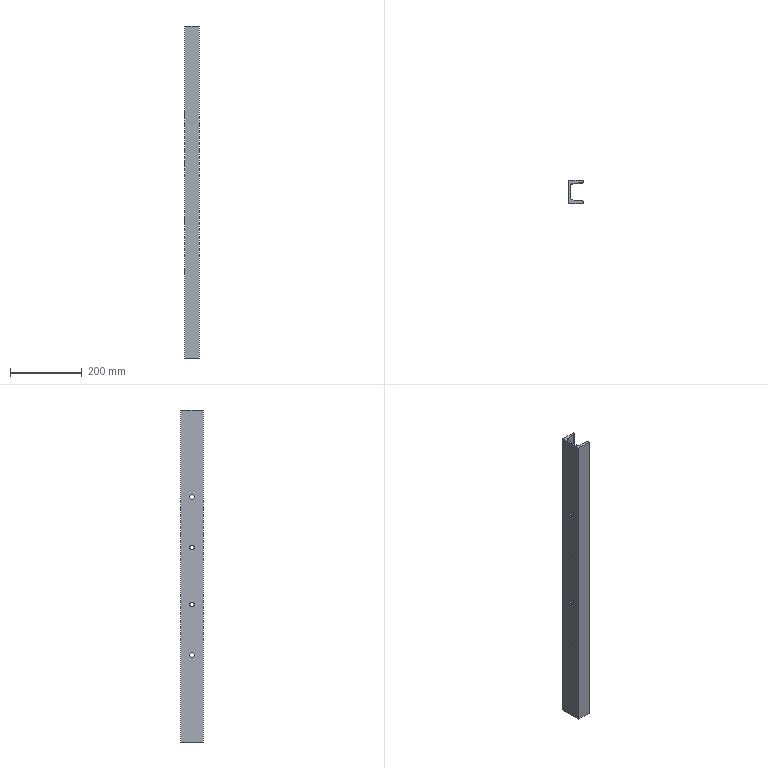Part | STEP file | 750038481 | 1 solid | 22 faces | box 40 x 63 x 924 mm | volume 778209 mm3 | cylinder 12 | plane 10 | commonest cylinder face diameters 12 x8 7.6 x2 15 x2
STEP:
#1=CARTESIAN_POINT('',(4.8,31.5,-86.));
#2=VERTEX_POINT('',#1);
#3=CARTESIAN_POINT('',(4.8,31.5,-74.));
#4=VERTEX_POINT('',#3);
#5=CARTESIAN_POINT('',(4.8,31.5,-80.));
#6=DIRECTION('',(-1.,0.,0.));
#7=DIRECTION('',(0.,0.,1.));
#8=AXIS2_PLACEMENT_3D('',#5,#6,#7);
#9=CIRCLE('',#8,6.);
#10=EDGE_CURVE('',#2,#4,#9,.T.);
#11=ORIENTED_EDGE('',*,*,#10,.F.);
#12=CARTESIAN_POINT('',(0.,31.5,-86.));
#13=VERTEX_POINT('',#12);
#14=CARTESIAN_POINT('',(279.,31.5,-86.));
#15=DIRECTION('',(-1.,0.,0.));
#16=VECTOR('',#15,1000.);
#17=LINE('',#14,#16);
#18=EDGE_CURVE('',#2,#13,#17,.T.);
#19=ORIENTED_EDGE('',*,*,#18,.T.);
#20=CARTESIAN_POINT('',(0.,31.5,-74.));
#21=VERTEX_POINT('',#20);
#22=CARTESIAN_POINT('',(0.,31.5,-80.));
#23=DIRECTION('',(-1.,0.,0.));
#24=DIRECTION('',(0.,0.,1.));
#25=AXIS2_PLACEMENT_3D('',#22,#23,#24);
#26=CIRCLE('',#25,6.);
#27=EDGE_CURVE('',#13,#21,#26,.T.);
#28=ORIENTED_EDGE('',*,*,#27,.T.);
#29=CARTESIAN_POINT('',(279.,31.5,-74.));
#30=DIRECTION('',(-1.,0.,0.));
#31=VECTOR('',#30,1000.);
#32=LINE('',#29,#31);
#33=EDGE_CURVE('',#4,#21,#32,.T.);
#34=ORIENTED_EDGE('',*,*,#33,.F.);
#35=EDGE_LOOP('',(#11,#19,#28,#34));
#36=FACE_OUTER_BOUND('',#35,.T.);
#37=CARTESIAN_POINT('',(279.,31.5,-80.));
#38=DIRECTION('',(-1.,0.,0.));
#39=DIRECTION('',(0.,0.,1.));
#40=AXIS2_PLACEMENT_3D('',#37,#38,#39);
#41=CYLINDRICAL_SURFACE('',#40,6.);
#42=ADVANCED_FACE('',(#36),#41,.F.);
#43=CARTESIAN_POINT('',(4.8,31.5,-226.));
#44=VERTEX_POINT('',#43);
#45=CARTESIAN_POINT('',(4.8,31.5,-214.));
#46=VERTEX_POINT('',#45);
#47=CARTESIAN_POINT('',(4.8,31.5,-220.));
#48=DIRECTION('',(-1.,0.,0.));
#49=DIRECTION('',(0.,0.,1.));
#50=AXIS2_PLACEMENT_3D('',#47,#48,#49);
#51=CIRCLE('',#50,6.);
#52=EDGE_CURVE('',#44,#46,#51,.T.);
#53=ORIENTED_EDGE('',*,*,#52,.F.);
#54=CARTESIAN_POINT('',(0.,31.5,-226.));
#55=VERTEX_POINT('',#54);
#56=CARTESIAN_POINT('',(279.,31.5,-226.));
#57=DIRECTION('',(-1.,0.,0.));
#58=VECTOR('',#57,1000.);
#59=LINE('',#56,#58);
#60=EDGE_CURVE('',#44,#55,#59,.T.);
#61=ORIENTED_EDGE('',*,*,#60,.T.);
#62=CARTESIAN_POINT('',(0.,31.5,-214.));
#63=VERTEX_POINT('',#62);
#64=CARTESIAN_POINT('',(0.,31.5,-220.));
#65=DIRECTION('',(-1.,0.,0.));
#66=DIRECTION('',(0.,0.,1.));
#67=AXIS2_PLACEMENT_3D('',#64,#65,#66);
#68=CIRCLE('',#67,6.);
#69=EDGE_CURVE('',#55,#63,#68,.T.);
#70=ORIENTED_EDGE('',*,*,#69,.T.);
#71=CARTESIAN_POINT('',(279.,31.5,-214.));
#72=DIRECTION('',(-1.,0.,0.));
#73=VECTOR('',#72,1000.);
#74=LINE('',#71,#73);
#75=EDGE_CURVE('',#46,#63,#74,.T.);
#76=ORIENTED_EDGE('',*,*,#75,.F.);
#77=EDGE_LOOP('',(#53,#61,#70,#76));
#78=FACE_OUTER_BOUND('',#77,.T.);
#79=CARTESIAN_POINT('',(279.,31.5,-220.));
#80=DIRECTION('',(-1.,0.,0.));
#81=DIRECTION('',(0.,0.,1.));
#82=AXIS2_PLACEMENT_3D('',#79,#80,#81);
#83=CYLINDRICAL_SURFACE('',#82,6.);
#84=ADVANCED_FACE('',(#78),#83,.F.);
#85=CARTESIAN_POINT('',(4.8,31.5,74.));
#86=VERTEX_POINT('',#85);
#87=CARTESIAN_POINT('',(4.8,31.5,86.));
#88=VERTEX_POINT('',#87);
#89=CARTESIAN_POINT('',(4.8,31.5,80.));
#90=DIRECTION('',(-1.,0.,0.));
#91=DIRECTION('',(0.,0.,1.));
#92=AXIS2_PLACEMENT_3D('',#89,#90,#91);
#93=CIRCLE('',#92,6.);
#94=EDGE_CURVE('',#86,#88,#93,.T.);
#95=ORIENTED_EDGE('',*,*,#94,.F.);
#96=CARTESIAN_POINT('',(0.,31.5,74.));
#97=VERTEX_POINT('',#96);
#98=CARTESIAN_POINT('',(279.,31.5,74.));
#99=DIRECTION('',(-1.,0.,0.));
#100=VECTOR('',#99,1000.);
#101=LINE('',#98,#100);
#102=EDGE_CURVE('',#86,#97,#101,.T.);
#103=ORIENTED_EDGE('',*,*,#102,.T.);
#104=CARTESIAN_POINT('',(0.,31.5,86.));
#105=VERTEX_POINT('',#104);
#106=CARTESIAN_POINT('',(0.,31.5,80.));
#107=DIRECTION('',(-1.,0.,0.));
#108=DIRECTION('',(0.,0.,1.));
#109=AXIS2_PLACEMENT_3D('',#106,#107,#108);
#110=CIRCLE('',#109,6.);
#111=EDGE_CURVE('',#97,#105,#110,.T.);
#112=ORIENTED_EDGE('',*,*,#111,.T.);
#113=CARTESIAN_POINT('',(279.,31.5,86.));
#114=DIRECTION('',(-1.,0.,0.));
#115=VECTOR('',#114,1000.);
#116=LINE('',#113,#115);
#117=EDGE_CURVE('',#88,#105,#116,.T.);
#118=ORIENTED_EDGE('',*,*,#117,.F.);
#119=EDGE_LOOP('',(#95,#103,#112,#118));
#120=FACE_OUTER_BOUND('',#119,.T.);
#121=CARTESIAN_POINT('',(279.,31.5,80.));
#122=DIRECTION('',(-1.,0.,0.));
#123=DIRECTION('',(0.,0.,1.));
#124=AXIS2_PLACEMENT_3D('',#121,#122,#123);
#125=CYLINDRICAL_SURFACE('',#124,6.);
#126=ADVANCED_FACE('',(#120),#125,.F.);
#127=CARTESIAN_POINT('',(4.8,31.5,214.));
#128=VERTEX_POINT('',#127);
#129=CARTESIAN_POINT('',(4.8,31.5,226.));
#130=VERTEX_POINT('',#129);
#131=CARTESIAN_POINT('',(4.8,31.5,220.));
#132=DIRECTION('',(-1.,0.,0.));
#133=DIRECTION('',(0.,0.,1.));
#134=AXIS2_PLACEMENT_3D('',#131,#132,#133);
#135=CIRCLE('',#134,6.);
#136=EDGE_CURVE('',#128,#130,#135,.T.);
#137=ORIENTED_EDGE('',*,*,#136,.F.);
#138=CARTESIAN_POINT('',(0.,31.5,214.));
#139=VERTEX_POINT('',#138);
#140=CARTESIAN_POINT('',(279.,31.5,214.));
#141=DIRECTION('',(-1.,0.,0.));
#142=VECTOR('',#141,1000.);
#143=LINE('',#140,#142);
#144=EDGE_CURVE('',#128,#139,#143,.T.);
#145=ORIENTED_EDGE('',*,*,#144,.T.);
#146=CARTESIAN_POINT('',(0.,31.5,226.));
#147=VERTEX_POINT('',#146);
#148=CARTESIAN_POINT('',(0.,31.5,220.));
#149=DIRECTION('',(-1.,0.,0.));
#150=DIRECTION('',(0.,0.,1.));
#151=AXIS2_PLACEMENT_3D('',#148,#149,#150);
#152=CIRCLE('',#151,6.);
#153=EDGE_CURVE('',#139,#147,#152,.T.);
#154=ORIENTED_EDGE('',*,*,#153,.T.);
#155=CARTESIAN_POINT('',(279.,31.5,226.));
#156=DIRECTION('',(-1.,0.,0.));
#157=VECTOR('',#156,1000.);
#158=LINE('',#155,#157);
#159=EDGE_CURVE('',#130,#147,#158,.T.);
#160=ORIENTED_EDGE('',*,*,#159,.F.);
#161=EDGE_LOOP('',(#137,#145,#154,#160));
#162=FACE_OUTER_BOUND('',#161,.T.);
#163=CARTESIAN_POINT('',(279.,31.5,220.));
#164=DIRECTION('',(-1.,0.,0.));
#165=DIRECTION('',(0.,0.,1.));
#166=AXIS2_PLACEMENT_3D('',#163,#164,#165);
#167=CYLINDRICAL_SURFACE('',#166,6.);
#168=ADVANCED_FACE('',(#162),#167,.F.);
#169=CARTESIAN_POINT('',(0.,31.5,-80.));
#170=DIRECTION('',(-1.,0.,0.));
#171=DIRECTION('',(0.,0.,1.));
#172=AXIS2_PLACEMENT_3D('',#169,#170,#171);
#173=CIRCLE('',#172,6.);
#174=EDGE_CURVE('',#21,#13,#173,.T.);
#175=ORIENTED_EDGE('',*,*,#174,.F.);
#176=ORIENTED_EDGE('',*,*,#27,.F.);
#177=EDGE_LOOP('',(#175,#176));
#178=FACE_BOUND('',#177,.T.);
#179=CARTESIAN_POINT('',(0.,31.5,-220.));
#180=DIRECTION('',(-1.,0.,0.));
#181=DIRECTION('',(0.,0.,1.));
#182=AXIS2_PLACEMENT_3D('',#179,#180,#181);
#183=CIRCLE('',#182,6.);
#184=EDGE_CURVE('',#63,#55,#183,.T.);
#185=ORIENTED_EDGE('',*,*,#184,.F.);
#186=ORIENTED_EDGE('',*,*,#69,.F.);
#187=EDGE_LOOP('',(#185,#186));
#188=FACE_BOUND('',#187,.T.);
#189=CARTESIAN_POINT('',(0.,0.,462.));
#190=VERTEX_POINT('',#189);
#191=CARTESIAN_POINT('',(0.,0.,-462.));
#192=VERTEX_POINT('',#191);
#193=CARTESIAN_POINT('',(0.,0.,462.));
#194=DIRECTION('',(0.,0.,-1.));
#195=VECTOR('',#194,1000.);
#196=LINE('',#193,#195);
#197=EDGE_CURVE('',#190,#192,#196,.T.);
#198=ORIENTED_EDGE('',*,*,#197,.F.);
#199=CARTESIAN_POINT('',(0.,63.,462.));
#200=VERTEX_POINT('',#199);
#201=CARTESIAN_POINT('',(0.,63.,462.));
#202=DIRECTION('',(0.,-1.,0.));
#203=VECTOR('',#202,1000.);
#204=LINE('',#201,#203);
#205=EDGE_CURVE('',#200,#190,#204,.T.);
#206=ORIENTED_EDGE('',*,*,#205,.F.);
#207=CARTESIAN_POINT('',(0.,63.,-462.));
#208=VERTEX_POINT('',#207);
#209=CARTESIAN_POINT('',(0.,63.,462.));
#210=DIRECTION('',(0.,0.,1.));
#211=VECTOR('',#210,1000.);
#212=LINE('',#209,#211);
#213=EDGE_CURVE('',#208,#200,#212,.T.);
#214=ORIENTED_EDGE('',*,*,#213,.F.);
#215=CARTESIAN_POINT('',(0.,63.,-462.));
#216=DIRECTION('',(0.,1.,0.));
#217=VECTOR('',#216,1000.);
#218=LINE('',#215,#217);
#219=EDGE_CURVE('',#192,#208,#218,.T.);
#220=ORIENTED_EDGE('',*,*,#219,.F.);
#221=EDGE_LOOP('',(#198,#206,#214,#220));
#222=FACE_OUTER_BOUND('',#221,.T.);
#223=CARTESIAN_POINT('',(0.,31.5,80.));
#224=DIRECTION('',(-1.,0.,0.));
#225=DIRECTION('',(0.,0.,1.));
#226=AXIS2_PLACEMENT_3D('',#223,#224,#225);
#227=CIRCLE('',#226,6.);
#228=EDGE_CURVE('',#105,#97,#227,.T.);
#229=ORIENTED_EDGE('',*,*,#228,.F.);
#230=ORIENTED_EDGE('',*,*,#111,.F.);
#231=EDGE_LOOP('',(#229,#230));
#232=FACE_BOUND('',#231,.T.);
#233=CARTESIAN_POINT('',(0.,31.5,220.));
#234=DIRECTION('',(-1.,0.,0.));
#235=DIRECTION('',(0.,0.,1.));
#236=AXIS2_PLACEMENT_3D('',#233,#234,#235);
#237=CIRCLE('',#236,6.);
#238=EDGE_CURVE('',#147,#139,#237,.T.);
#239=ORIENTED_EDGE('',*,*,#238,.F.);
#240=ORIENTED_EDGE('',*,*,#153,.F.);
#241=EDGE_LOOP('',(#239,#240));
#242=FACE_BOUND('',#241,.T.);
#243=CARTESIAN_POINT('',(0.,63.,462.));
#244=DIRECTION('',(1.,0.,0.));
#245=DIRECTION('',(0.,0.,-1.));
#246=AXIS2_PLACEMENT_3D('',#243,#244,#245);
#247=PLANE('',#246);
#248=ADVANCED_FACE('',(#178,#188,#222,#232,#242),#247,.F.);
#249=ORIENTED_EDGE('',*,*,#18,.F.);
#250=CARTESIAN_POINT('',(4.8,31.5,-80.));
#251=DIRECTION('',(-1.,0.,0.));
#252=DIRECTION('',(0.,0.,1.));
#253=AXIS2_PLACEMENT_3D('',#250,#251,#252);
#254=CIRCLE('',#253,6.);
#255=EDGE_CURVE('',#4,#2,#254,.T.);
#256=ORIENTED_EDGE('',*,*,#255,.F.);
#257=ORIENTED_EDGE('',*,*,#33,.T.);
#258=ORIENTED_EDGE('',*,*,#174,.T.);
#259=EDGE_LOOP('',(#249,#256,#257,#258));
#260=FACE_OUTER_BOUND('',#259,.T.);
#261=CARTESIAN_POINT('',(279.,31.5,-80.));
#262=DIRECTION('',(-1.,0.,0.));
#263=DIRECTION('',(0.,0.,1.));
#264=AXIS2_PLACEMENT_3D('',#261,#262,#263);
#265=CYLINDRICAL_SURFACE('',#264,6.);
#266=ADVANCED_FACE('',(#260),#265,.F.);
#267=ORIENTED_EDGE('',*,*,#60,.F.);
#268=CARTESIAN_POINT('',(4.8,31.5,-220.));
#269=DIRECTION('',(-1.,0.,0.));
#270=DIRECTION('',(0.,0.,1.));
#271=AXIS2_PLACEMENT_3D('',#268,#269,#270);
#272=CIRCLE('',#271,6.);
#273=EDGE_CURVE('',#46,#44,#272,.T.);
#274=ORIENTED_EDGE('',*,*,#273,.F.);
#275=ORIENTED_EDGE('',*,*,#75,.T.);
#276=ORIENTED_EDGE('',*,*,#184,.T.);
#277=EDGE_LOOP('',(#267,#274,#275,#276));
#278=FACE_OUTER_BOUND('',#277,.T.);
#279=CARTESIAN_POINT('',(279.,31.5,-220.));
#280=DIRECTION('',(-1.,0.,0.));
#281=DIRECTION('',(0.,0.,1.));
#282=AXIS2_PLACEMENT_3D('',#279,#280,#281);
#283=CYLINDRICAL_SURFACE('',#282,6.);
#284=ADVANCED_FACE('',(#278),#283,.F.);
#285=CARTESIAN_POINT('',(40.,63.,-462.));
#286=VERTEX_POINT('',#285);
#287=CARTESIAN_POINT('',(36.2,63.,-462.));
#288=DIRECTION('',(-1.,0.,0.));
#289=VECTOR('',#288,1000.);
#290=LINE('',#287,#289);
#291=EDGE_CURVE('',#286,#208,#290,.T.);
#292=ORIENTED_EDGE('',*,*,#291,.F.);
#293=CARTESIAN_POINT('',(40.,60.699,-462.));
#294=VERTEX_POINT('',#293);
#295=CARTESIAN_POINT('',(40.,2.301,-462.));
#296=DIRECTION('',(0.,1.,0.));
#297=VECTOR('',#296,1000.);
#298=LINE('',#295,#297);
#299=EDGE_CURVE('',#294,#286,#298,.T.);
#300=ORIENTED_EDGE('',*,*,#299,.F.);
#301=CARTESIAN_POINT('',(36.578,56.918,-462.));
#302=VERTEX_POINT('',#301);
#303=CARTESIAN_POINT('',(36.2,60.699,-462.));
#304=DIRECTION('',(0.,0.,1.));
#305=DIRECTION('',(-1.,0.,0.));
#306=AXIS2_PLACEMENT_3D('',#303,#304,#305);
#307=CIRCLE('',#306,3.8);
#308=EDGE_CURVE('',#302,#294,#307,.T.);
#309=ORIENTED_EDGE('',*,*,#308,.F.);
#310=CARTESIAN_POINT('',(11.554,54.415,-462.));
#311=VERTEX_POINT('',#310);
#312=CARTESIAN_POINT('',(11.554,54.415,-462.));
#313=DIRECTION('',(0.995,0.0995,0.));
#314=VECTOR('',#313,1000.);
#315=LINE('',#312,#314);
#316=EDGE_CURVE('',#311,#302,#315,.T.);
#317=ORIENTED_EDGE('',*,*,#316,.F.);
#318=CARTESIAN_POINT('',(4.8,46.953,-462.));
#319=VERTEX_POINT('',#318);
#320=CARTESIAN_POINT('',(12.3,46.953,-462.));
#321=DIRECTION('',(0.,0.,-1.));
#322=DIRECTION('',(-1.,0.,0.));
#323=AXIS2_PLACEMENT_3D('',#320,#321,#322);
#324=CIRCLE('',#323,7.5);
#325=EDGE_CURVE('',#319,#311,#324,.T.);
#326=ORIENTED_EDGE('',*,*,#325,.F.);
#327=CARTESIAN_POINT('',(4.8,16.047,-462.));
#328=VERTEX_POINT('',#327);
#329=CARTESIAN_POINT('',(4.8,2.301,-462.));
#330=DIRECTION('',(0.,1.,0.));
#331=VECTOR('',#330,1000.);
#332=LINE('',#329,#331);
#333=EDGE_CURVE('',#328,#319,#332,.T.);
#334=ORIENTED_EDGE('',*,*,#333,.F.);
#335=CARTESIAN_POINT('',(11.554,8.585,-462.));
#336=VERTEX_POINT('',#335);
#337=CARTESIAN_POINT('',(12.3,16.047,-462.));
#338=DIRECTION('',(0.,0.,-1.));
#339=DIRECTION('',(-1.,0.,0.));
#340=AXIS2_PLACEMENT_3D('',#337,#338,#339);
#341=CIRCLE('',#340,7.5);
#342=EDGE_CURVE('',#336,#328,#341,.T.);
#343=ORIENTED_EDGE('',*,*,#342,.F.);
#344=CARTESIAN_POINT('',(36.578,6.082,-462.));
#345=VERTEX_POINT('',#344);
#346=CARTESIAN_POINT('',(36.578,6.082,-462.));
#347=DIRECTION('',(-0.995,0.0995,0.));
#348=VECTOR('',#347,1000.);
#349=LINE('',#346,#348);
#350=EDGE_CURVE('',#345,#336,#349,.T.);
#351=ORIENTED_EDGE('',*,*,#350,.F.);
#352=CARTESIAN_POINT('',(40.,2.301,-462.));
#353=VERTEX_POINT('',#352);
#354=CARTESIAN_POINT('',(36.2,2.301,-462.));
#355=DIRECTION('',(0.,0.,1.));
#356=DIRECTION('',(-1.,0.,0.));
#357=AXIS2_PLACEMENT_3D('',#354,#355,#356);
#358=CIRCLE('',#357,3.8);
#359=EDGE_CURVE('',#353,#345,#358,.T.);
#360=ORIENTED_EDGE('',*,*,#359,.F.);
#361=CARTESIAN_POINT('',(40.,0.,-462.));
#362=VERTEX_POINT('',#361);
#363=CARTESIAN_POINT('',(40.,2.301,-462.));
#364=DIRECTION('',(0.,1.,0.));
#365=VECTOR('',#364,1000.);
#366=LINE('',#363,#365);
#367=EDGE_CURVE('',#362,#353,#366,.T.);
#368=ORIENTED_EDGE('',*,*,#367,.F.);
#369=CARTESIAN_POINT('',(36.2,0.,-462.));
#370=DIRECTION('',(1.,0.,0.));
#371=VECTOR('',#370,1000.);
#372=LINE('',#369,#371);
#373=EDGE_CURVE('',#192,#362,#372,.T.);
#374=ORIENTED_EDGE('',*,*,#373,.F.);
#375=ORIENTED_EDGE('',*,*,#219,.T.);
#376=EDGE_LOOP('',(#292,#300,#309,#317,#326,#334,#343,#351,#360,#368,#374,#375));
#377=FACE_OUTER_BOUND('',#376,.T.);
#378=CARTESIAN_POINT('',(36.2,2.301,-462.));
#379=DIRECTION('',(0.,0.,1.));
#380=DIRECTION('',(1.,0.,0.));
#381=AXIS2_PLACEMENT_3D('',#378,#379,#380);
#382=PLANE('',#381);
#383=ADVANCED_FACE('',(#377),#382,.F.);
#384=CARTESIAN_POINT('',(40.,0.,462.));
#385=VERTEX_POINT('',#384);
#386=CARTESIAN_POINT('',(40.,0.,462.));
#387=DIRECTION('',(0.,0.,-1.));
#388=VECTOR('',#387,1000.);
#389=LINE('',#386,#388);
#390=EDGE_CURVE('',#385,#362,#389,.T.);
#391=ORIENTED_EDGE('',*,*,#390,.F.);
#392=CARTESIAN_POINT('',(0.,0.,462.));
#393=DIRECTION('',(1.,0.,0.));
#394=VECTOR('',#393,1000.);
#395=LINE('',#392,#394);
#396=EDGE_CURVE('',#190,#385,#395,.T.);
#397=ORIENTED_EDGE('',*,*,#396,.F.);
#398=ORIENTED_EDGE('',*,*,#197,.T.);
#399=ORIENTED_EDGE('',*,*,#373,.T.);
#400=EDGE_LOOP('',(#391,#397,#398,#399));
#401=FACE_OUTER_BOUND('',#400,.T.);
#402=CARTESIAN_POINT('',(0.,0.,462.));
#403=DIRECTION('',(0.,1.,0.));
#404=DIRECTION('',(0.,0.,1.));
#405=AXIS2_PLACEMENT_3D('',#402,#403,#404);
#406=PLANE('',#405);
#407=ADVANCED_FACE('',(#401),#406,.F.);
#408=CARTESIAN_POINT('',(40.,60.699,462.));
#409=VERTEX_POINT('',#408);
#410=CARTESIAN_POINT('',(40.,63.,462.));
#411=VERTEX_POINT('',#410);
#412=CARTESIAN_POINT('',(40.,2.301,462.));
#413=DIRECTION('',(0.,1.,0.));
#414=VECTOR('',#413,1000.);
#415=LINE('',#412,#414);
#416=EDGE_CURVE('',#409,#411,#415,.T.);
#417=ORIENTED_EDGE('',*,*,#416,.T.);
#418=CARTESIAN_POINT('',(36.2,63.,462.));
#419=DIRECTION('',(-1.,0.,0.));
#420=VECTOR('',#419,1000.);
#421=LINE('',#418,#420);
#422=EDGE_CURVE('',#411,#200,#421,.T.);
#423=ORIENTED_EDGE('',*,*,#422,.T.);
#424=ORIENTED_EDGE('',*,*,#205,.T.);
#425=ORIENTED_EDGE('',*,*,#396,.T.);
#426=CARTESIAN_POINT('',(40.,2.301,462.));
#427=VERTEX_POINT('',#426);
#428=CARTESIAN_POINT('',(40.,2.301,462.));
#429=DIRECTION('',(0.,1.,0.));
#430=VECTOR('',#429,1000.);
#431=LINE('',#428,#430);
#432=EDGE_CURVE('',#385,#427,#431,.T.);
#433=ORIENTED_EDGE('',*,*,#432,.T.);
#434=CARTESIAN_POINT('',(36.578,6.082,462.));
#435=VERTEX_POINT('',#434);
#436=CARTESIAN_POINT('',(36.2,2.301,462.));
#437=DIRECTION('',(0.,0.,1.));
#438=DIRECTION('',(-1.,0.,0.));
#439=AXIS2_PLACEMENT_3D('',#436,#437,#438);
#440=CIRCLE('',#439,3.8);
#441=EDGE_CURVE('',#427,#435,#440,.T.);
#442=ORIENTED_EDGE('',*,*,#441,.T.);
#443=CARTESIAN_POINT('',(11.554,8.585,462.));
#444=VERTEX_POINT('',#443);
#445=CARTESIAN_POINT('',(36.578,6.082,462.));
#446=DIRECTION('',(-0.995,0.0995,0.));
#447=VECTOR('',#446,1000.);
#448=LINE('',#445,#447);
#449=EDGE_CURVE('',#435,#444,#448,.T.);
#450=ORIENTED_EDGE('',*,*,#449,.T.);
#451=CARTESIAN_POINT('',(4.8,16.047,462.));
#452=VERTEX_POINT('',#451);
#453=CARTESIAN_POINT('',(12.3,16.047,462.));
#454=DIRECTION('',(0.,0.,-1.));
#455=DIRECTION('',(-1.,0.,0.));
#456=AXIS2_PLACEMENT_3D('',#453,#454,#455);
#457=CIRCLE('',#456,7.5);
#458=EDGE_CURVE('',#444,#452,#457,.T.);
#459=ORIENTED_EDGE('',*,*,#458,.T.);
#460=CARTESIAN_POINT('',(4.8,46.953,462.));
#461=VERTEX_POINT('',#460);
#462=CARTESIAN_POINT('',(4.8,2.301,462.));
#463=DIRECTION('',(0.,1.,0.));
#464=VECTOR('',#463,1000.);
#465=LINE('',#462,#464);
#466=EDGE_CURVE('',#452,#461,#465,.T.);
#467=ORIENTED_EDGE('',*,*,#466,.T.);
#468=CARTESIAN_POINT('',(11.554,54.415,462.));
#469=VERTEX_POINT('',#468);
#470=CARTESIAN_POINT('',(12.3,46.953,462.));
#471=DIRECTION('',(0.,0.,-1.));
#472=DIRECTION('',(-1.,0.,0.));
#473=AXIS2_PLACEMENT_3D('',#470,#471,#472);
#474=CIRCLE('',#473,7.5);
#475=EDGE_CURVE('',#461,#469,#474,.T.);
#476=ORIENTED_EDGE('',*,*,#475,.T.);
#477=CARTESIAN_POINT('',(36.578,56.918,462.));
#478=VERTEX_POINT('',#477);
#479=CARTESIAN_POINT('',(11.554,54.415,462.));
#480=DIRECTION('',(0.995,0.0995,0.));
#481=VECTOR('',#480,1000.);
#482=LINE('',#479,#481);
#483=EDGE_CURVE('',#469,#478,#482,.T.);
#484=ORIENTED_EDGE('',*,*,#483,.T.);
#485=CARTESIAN_POINT('',(36.2,60.699,462.));
#486=DIRECTION('',(0.,0.,1.));
#487=DIRECTION('',(-1.,0.,0.));
#488=AXIS2_PLACEMENT_3D('',#485,#486,#487);
#489=CIRCLE('',#488,3.8);
#490=EDGE_CURVE('',#478,#409,#489,.T.);
#491=ORIENTED_EDGE('',*,*,#490,.T.);
#492=EDGE_LOOP('',(#417,#423,#424,#425,#433,#442,#450,#459,#467,#476,#484,#491));
#493=FACE_OUTER_BOUND('',#492,.T.);
#494=CARTESIAN_POINT('',(36.2,2.301,462.));
#495=DIRECTION('',(0.,0.,1.));
#496=DIRECTION('',(1.,0.,0.));
#497=AXIS2_PLACEMENT_3D('',#494,#495,#496);
#498=PLANE('',#497);
#499=ADVANCED_FACE('',(#493),#498,.T.);
#500=ORIENTED_EDGE('',*,*,#213,.T.);
#501=ORIENTED_EDGE('',*,*,#422,.F.);
#502=CARTESIAN_POINT('',(40.,63.,462.));
#503=DIRECTION('',(0.,0.,1.));
#504=VECTOR('',#503,1000.);
#505=LINE('',#502,#504);
#506=EDGE_CURVE('',#286,#411,#505,.T.);
#507=ORIENTED_EDGE('',*,*,#506,.F.);
#508=ORIENTED_EDGE('',*,*,#291,.T.);
#509=EDGE_LOOP('',(#500,#501,#507,#508));
#510=FACE_OUTER_BOUND('',#509,.T.);
#511=CARTESIAN_POINT('',(40.,63.,462.));
#512=DIRECTION('',(0.,-1.,0.));
#513=DIRECTION('',(0.,0.,-1.));
#514=AXIS2_PLACEMENT_3D('',#511,#512,#513);
#515=PLANE('',#514);
#516=ADVANCED_FACE('',(#510),#515,.F.);
#517=ORIENTED_EDGE('',*,*,#102,.F.);
#518=CARTESIAN_POINT('',(4.8,31.5,80.));
#519=DIRECTION('',(-1.,0.,0.));
#520=DIRECTION('',(0.,0.,1.));
#521=AXIS2_PLACEMENT_3D('',#518,#519,#520);
#522=CIRCLE('',#521,6.);
#523=EDGE_CURVE('',#88,#86,#522,.T.);
#524=ORIENTED_EDGE('',*,*,#523,.F.);
#525=ORIENTED_EDGE('',*,*,#117,.T.);
#526=ORIENTED_EDGE('',*,*,#228,.T.);
#527=EDGE_LOOP('',(#517,#524,#525,#526));
#528=FACE_OUTER_BOUND('',#527,.T.);
#529=CARTESIAN_POINT('',(279.,31.5,80.));
#530=DIRECTION('',(-1.,0.,0.));
#531=DIRECTION('',(0.,0.,1.));
#532=AXIS2_PLACEMENT_3D('',#529,#530,#531);
#533=CYLINDRICAL_SURFACE('',#532,6.);
#534=ADVANCED_FACE('',(#528),#533,.F.);
#535=ORIENTED_EDGE('',*,*,#144,.F.);
#536=CARTESIAN_POINT('',(4.8,31.5,220.));
#537=DIRECTION('',(-1.,0.,0.));
#538=DIRECTION('',(0.,0.,1.));
#539=AXIS2_PLACEMENT_3D('',#536,#537,#538);
#540=CIRCLE('',#539,6.);
#541=EDGE_CURVE('',#130,#128,#540,.T.);
#542=ORIENTED_EDGE('',*,*,#541,.F.);
#543=ORIENTED_EDGE('',*,*,#159,.T.);
#544=ORIENTED_EDGE('',*,*,#238,.T.);
#545=EDGE_LOOP('',(#535,#542,#543,#544));
#546=FACE_OUTER_BOUND('',#545,.T.);
#547=CARTESIAN_POINT('',(279.,31.5,220.));
#548=DIRECTION('',(-1.,0.,0.));
#549=DIRECTION('',(0.,0.,1.));
#550=AXIS2_PLACEMENT_3D('',#547,#548,#549);
#551=CYLINDRICAL_SURFACE('',#550,6.);
#552=ADVANCED_FACE('',(#546),#551,.F.);
#553=ORIENTED_EDGE('',*,*,#255,.T.);
#554=ORIENTED_EDGE('',*,*,#10,.T.);
#555=EDGE_LOOP('',(#553,#554));
#556=FACE_BOUND('',#555,.T.);
#557=CARTESIAN_POINT('',(4.8,46.953,462.));
#558=DIRECTION('',(0.,0.,-1.));
#559=VECTOR('',#558,1000.);
#560=LINE('',#557,#559);
#561=EDGE_CURVE('',#461,#319,#560,.T.);
#562=ORIENTED_EDGE('',*,*,#561,.F.);
#563=ORIENTED_EDGE('',*,*,#466,.F.);
#564=CARTESIAN_POINT('',(4.8,16.047,462.));
#565=DIRECTION('',(0.,0.,1.));
#566=VECTOR('',#565,1000.);
#567=LINE('',#564,#566);
#568=EDGE_CURVE('',#328,#452,#567,.T.);
#569=ORIENTED_EDGE('',*,*,#568,.F.);
#570=ORIENTED_EDGE('',*,*,#333,.T.);
#571=EDGE_LOOP('',(#562,#563,#569,#570));
#572=FACE_OUTER_BOUND('',#571,.T.);
#573=ORIENTED_EDGE('',*,*,#523,.T.);
#574=ORIENTED_EDGE('',*,*,#94,.T.);
#575=EDGE_LOOP('',(#573,#574));
#576=FACE_BOUND('',#575,.T.);
#577=ORIENTED_EDGE('',*,*,#273,.T.);
#578=ORIENTED_EDGE('',*,*,#52,.T.);
#579=EDGE_LOOP('',(#577,#578));
#580=FACE_BOUND('',#579,.T.);
#581=ORIENTED_EDGE('',*,*,#541,.T.);
#582=ORIENTED_EDGE('',*,*,#136,.T.);
#583=EDGE_LOOP('',(#581,#582));
#584=FACE_BOUND('',#583,.T.);
#585=CARTESIAN_POINT('',(4.8,16.047,462.));
#586=DIRECTION('',(-1.,0.,0.));
#587=DIRECTION('',(0.,-1.,0.));
#588=AXIS2_PLACEMENT_3D('',#585,#586,#587);
#589=PLANE('',#588);
#590=ADVANCED_FACE('',(#556,#572,#576,#580,#584),#589,.F.);
#591=ORIENTED_EDGE('',*,*,#506,.T.);
#592=ORIENTED_EDGE('',*,*,#416,.F.);
#593=CARTESIAN_POINT('',(40.,60.699,462.));
#594=DIRECTION('',(0.,0.,1.));
#595=VECTOR('',#594,1000.);
#596=LINE('',#593,#595);
#597=EDGE_CURVE('',#294,#409,#596,.T.);
#598=ORIENTED_EDGE('',*,*,#597,.F.);
#599=ORIENTED_EDGE('',*,*,#299,.T.);
#600=EDGE_LOOP('',(#591,#592,#598,#599));
#601=FACE_OUTER_BOUND('',#600,.T.);
#602=CARTESIAN_POINT('',(40.,60.699,462.));
#603=DIRECTION('',(-1.,0.,0.));
#604=DIRECTION('',(0.,-1.,0.));
#605=AXIS2_PLACEMENT_3D('',#602,#603,#604);
#606=PLANE('',#605);
#607=ADVANCED_FACE('',(#601),#606,.F.);
#608=ORIENTED_EDGE('',*,*,#490,.F.);
#609=CARTESIAN_POINT('',(36.578,56.918,462.));
#610=DIRECTION('',(0.,0.,-1.));
#611=VECTOR('',#610,1000.);
#612=LINE('',#609,#611);
#613=EDGE_CURVE('',#478,#302,#612,.T.);
#614=ORIENTED_EDGE('',*,*,#613,.T.);
#615=ORIENTED_EDGE('',*,*,#308,.T.);
#616=ORIENTED_EDGE('',*,*,#597,.T.);
#617=EDGE_LOOP('',(#608,#614,#615,#616));
#618=FACE_OUTER_BOUND('',#617,.T.);
#619=CARTESIAN_POINT('',(36.2,60.699,462.));
#620=DIRECTION('',(0.,0.,-1.));
#621=DIRECTION('',(-1.,0.,0.));
#622=AXIS2_PLACEMENT_3D('',#619,#620,#621);
#623=CYLINDRICAL_SURFACE('',#622,3.8);
#624=ADVANCED_FACE('',(#618),#623,.T.);
#625=ORIENTED_EDGE('',*,*,#613,.F.);
#626=ORIENTED_EDGE('',*,*,#483,.F.);
#627=CARTESIAN_POINT('',(11.554,54.415,462.));
#628=DIRECTION('',(0.,0.,1.));
#629=VECTOR('',#628,1000.);
#630=LINE('',#627,#629);
#631=EDGE_CURVE('',#311,#469,#630,.T.);
#632=ORIENTED_EDGE('',*,*,#631,.F.);
#633=ORIENTED_EDGE('',*,*,#316,.T.);
#634=EDGE_LOOP('',(#625,#626,#632,#633));
#635=FACE_OUTER_BOUND('',#634,.T.);
#636=CARTESIAN_POINT('',(11.554,54.415,462.));
#637=DIRECTION('',(-0.0995,0.995,0.));
#638=DIRECTION('',(-0.995,-0.0995,0.));
#639=AXIS2_PLACEMENT_3D('',#636,#637,#638);
#640=PLANE('',#639);
#641=ADVANCED_FACE('',(#635),#640,.F.);
#642=ORIENTED_EDGE('',*,*,#631,.T.);
#643=ORIENTED_EDGE('',*,*,#475,.F.);
#644=ORIENTED_EDGE('',*,*,#561,.T.);
#645=ORIENTED_EDGE('',*,*,#325,.T.);
#646=EDGE_LOOP('',(#642,#643,#644,#645));
#647=FACE_OUTER_BOUND('',#646,.T.);
#648=CARTESIAN_POINT('',(12.3,46.953,462.));
#649=DIRECTION('',(0.,0.,-1.));
#650=DIRECTION('',(-1.,0.,0.));
#651=AXIS2_PLACEMENT_3D('',#648,#649,#650);
#652=CYLINDRICAL_SURFACE('',#651,7.5);
#653=ADVANCED_FACE('',(#647),#652,.F.);
#654=ORIENTED_EDGE('',*,*,#568,.T.);
#655=ORIENTED_EDGE('',*,*,#458,.F.);
#656=CARTESIAN_POINT('',(11.554,8.585,462.));
#657=DIRECTION('',(0.,0.,1.));
#658=VECTOR('',#657,1000.);
#659=LINE('',#656,#658);
#660=EDGE_CURVE('',#336,#444,#659,.T.);
#661=ORIENTED_EDGE('',*,*,#660,.F.);
#662=ORIENTED_EDGE('',*,*,#342,.T.);
#663=EDGE_LOOP('',(#654,#655,#661,#662));
#664=FACE_OUTER_BOUND('',#663,.T.);
#665=CARTESIAN_POINT('',(12.3,16.047,462.));
#666=DIRECTION('',(0.,0.,-1.));
#667=DIRECTION('',(-1.,0.,0.));
#668=AXIS2_PLACEMENT_3D('',#665,#666,#667);
#669=CYLINDRICAL_SURFACE('',#668,7.5);
#670=ADVANCED_FACE('',(#664),#669,.F.);
#671=ORIENTED_EDGE('',*,*,#660,.T.);
#672=ORIENTED_EDGE('',*,*,#449,.F.);
#673=CARTESIAN_POINT('',(36.578,6.082,462.));
#674=DIRECTION('',(0.,0.,1.));
#675=VECTOR('',#674,1000.);
#676=LINE('',#673,#675);
#677=EDGE_CURVE('',#345,#435,#676,.T.);
#678=ORIENTED_EDGE('',*,*,#677,.F.);
#679=ORIENTED_EDGE('',*,*,#350,.T.);
#680=EDGE_LOOP('',(#671,#672,#678,#679));
#681=FACE_OUTER_BOUND('',#680,.T.);
#682=CARTESIAN_POINT('',(36.578,6.082,462.));
#683=DIRECTION('',(-0.0995,-0.995,0.));
#684=DIRECTION('',(0.995,-0.0995,0.));
#685=AXIS2_PLACEMENT_3D('',#682,#683,#684);
#686=PLANE('',#685);
#687=ADVANCED_FACE('',(#681),#686,.F.);
#688=ORIENTED_EDGE('',*,*,#441,.F.);
#689=CARTESIAN_POINT('',(40.,2.301,462.));
#690=DIRECTION('',(0.,0.,-1.));
#691=VECTOR('',#690,1000.);
#692=LINE('',#689,#691);
#693=EDGE_CURVE('',#427,#353,#692,.T.);
#694=ORIENTED_EDGE('',*,*,#693,.T.);
#695=ORIENTED_EDGE('',*,*,#359,.T.);
#696=ORIENTED_EDGE('',*,*,#677,.T.);
#697=EDGE_LOOP('',(#688,#694,#695,#696));
#698=FACE_OUTER_BOUND('',#697,.T.);
#699=CARTESIAN_POINT('',(36.2,2.301,462.));
#700=DIRECTION('',(0.,0.,-1.));
#701=DIRECTION('',(-1.,0.,0.));
#702=AXIS2_PLACEMENT_3D('',#699,#700,#701);
#703=CYLINDRICAL_SURFACE('',#702,3.8);
#704=ADVANCED_FACE('',(#698),#703,.T.);
#705=ORIENTED_EDGE('',*,*,#693,.F.);
#706=ORIENTED_EDGE('',*,*,#432,.F.);
#707=ORIENTED_EDGE('',*,*,#390,.T.);
#708=ORIENTED_EDGE('',*,*,#367,.T.);
#709=EDGE_LOOP('',(#705,#706,#707,#708));
#710=FACE_OUTER_BOUND('',#709,.T.);
#711=CARTESIAN_POINT('',(40.,0.,462.));
#712=DIRECTION('',(-1.,0.,0.));
#713=DIRECTION('',(0.,0.,1.));
#714=AXIS2_PLACEMENT_3D('',#711,#712,#713);
#715=PLANE('',#714);
#716=ADVANCED_FACE('',(#710),#715,.F.);
#717=CLOSED_SHELL('',(#42,#84,#126,#168,#248,#266,#284,#383,#407,#499,#516,#534,#552,#590,#607,#624,#641,#653,#670,#687,#704,#716));
#718=MANIFOLD_SOLID_BREP('',#717);
#719=CARTESIAN_POINT('',(0.,0.,0.));
#720=DIRECTION('',(0.,0.,1.));
#721=DIRECTION('',(1.,0.,0.));
#722=AXIS2_PLACEMENT_3D('',#719,#720,#721);
#723=(LENGTH_UNIT()NAMED_UNIT(*)SI_UNIT(.MILLI.,.METRE.));
#724=UNCERTAINTY_MEASURE_WITH_UNIT(LENGTH_MEASURE(0.00001),#723,'','');
#725=(NAMED_UNIT(*)PLANE_ANGLE_UNIT()SI_UNIT($,.RADIAN.));
#726=(NAMED_UNIT(*)SI_UNIT($,.STERADIAN.)SOLID_ANGLE_UNIT());
#727=(GEOMETRIC_REPRESENTATION_CONTEXT(3)GLOBAL_UNCERTAINTY_ASSIGNED_CONTEXT((#724))GLOBAL_UNIT_ASSIGNED_CONTEXT((#723,#725,#726))REPRESENTATION_CONTEXT('',''));
#728=ADVANCED_BREP_SHAPE_REPRESENTATION('',(#718,#722),#727);